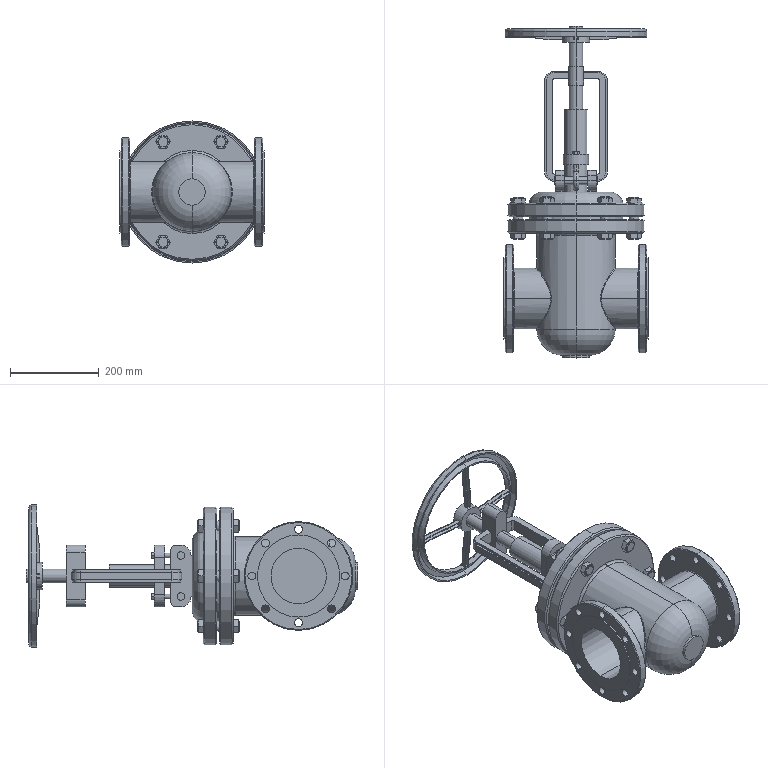Part | SolidWorks | features BaseBody 1 | 1 solid | 678 faces | box 325 x 747.833 x 320 mm | volume 15071073 mm3 | plane 263 | cylinder 225 | cone 148 | torus 38 | spline 4 | commonest cylinder face diameters 22.849 x36 18 x32 7.418 x24 17.387 x12 272 x9 10.432 x8